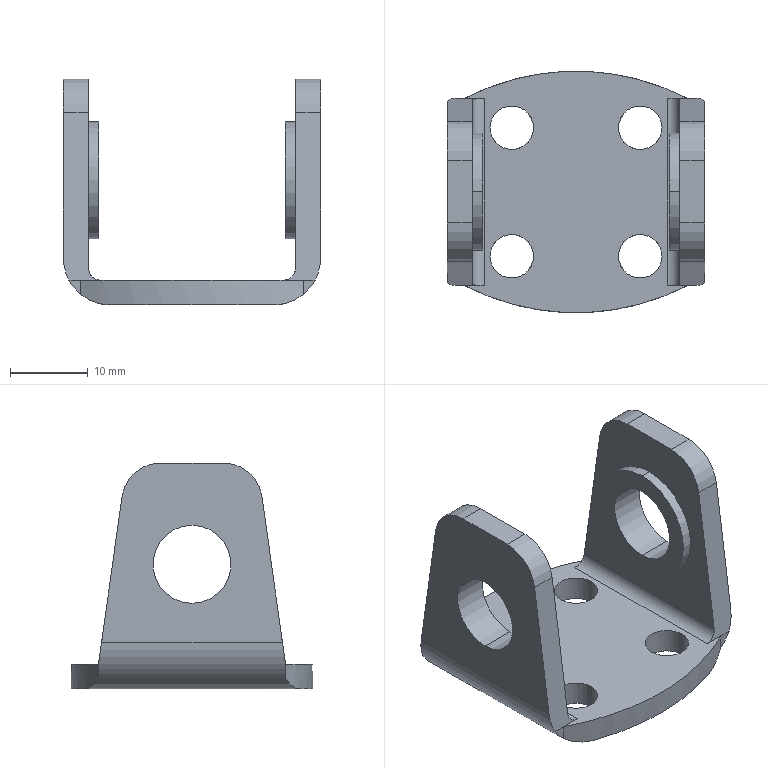Part | STEP file | 0229_Z_Cylinder_CG1DN25-75_4 | 1 solid | 47 faces | box 33 x 31 x 29 mm | volume 5061 mm3 | cylinder 28 | plane 19 | commonest cylinder face diameters 5.6 x8 10 x8 15 x4 3 x2 12 x2 14 x2